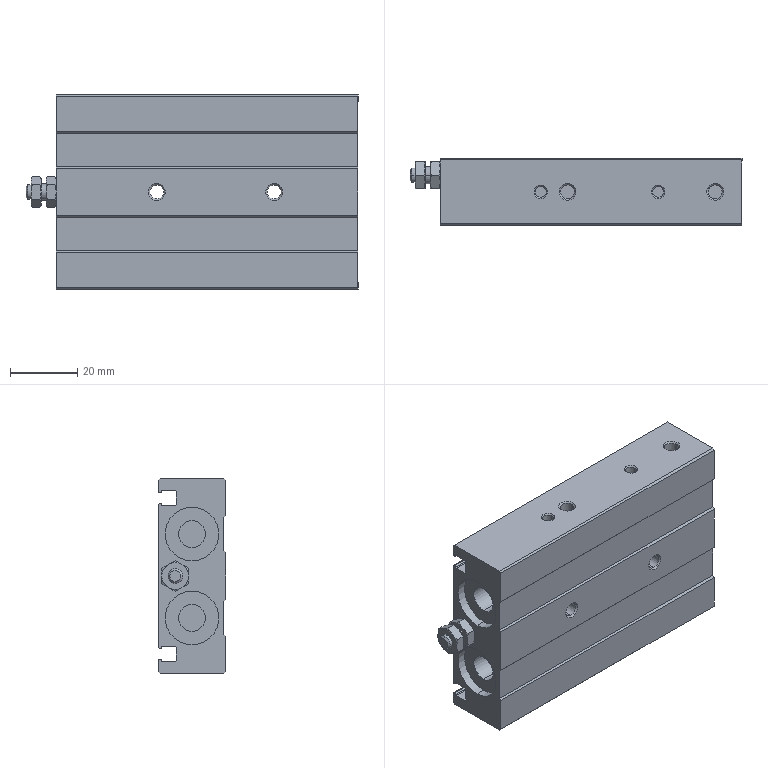Part | SolidWorks | features BaseBody 1 | 1 solid | 189 faces | box 99 x 20 x 58 mm | volume 74621 mm3 | cylinder 68 | plane 68 | cone 53 | commonest cylinder face diameters 0.8 x12 4.134 x12 3.242 x8 8 x8 16 x8 0.4 x4